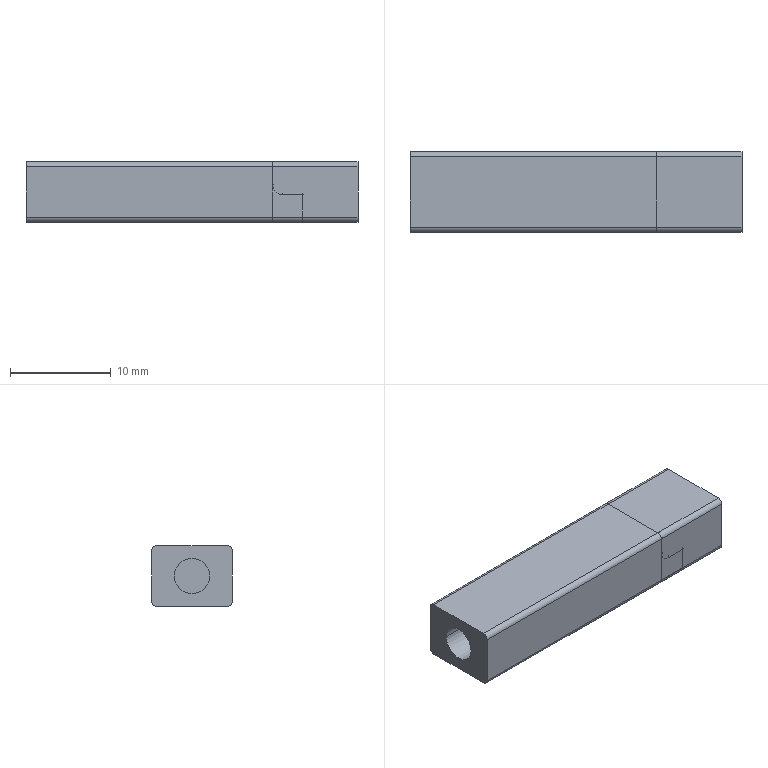NC program | NX | posted with a generic post | part box 33 x 8 x 6 mm
Lines 1 to 1894 of 11867, first 1555 of 1876 lines:
N10 G17 G21 G94 G90
(CAVITY_MILL_COPY , TOOL : D4)
N12 T04 M6
N14 G54
N16 G17 G0 G90 X2.078 Y5.8 B0. C0. S9500 M3
N18 G43 Z30. H4
N20 Z-0.445
N22 G94 G1 X0.866 Y3.7 F1000.
N24 G2 X0. Y3.2 R1.
N26 G1 X-3.5 F2000.
N28 G3 X-4.2 Y2.5 R0.7
N30 G1 Y-2.5
N32 G3 X-3.5 Y-3.2 R0.7
N34 G1 X-3.093
N36 G3 X-0.373 Y-4.42 R3.658
N38 X0.205 Y-5. R3.158
N40 G1 X1.429
N42 G2 X-0.087 Y-3.847 R2.598
N44 X2.14 Y1.058 R-3.098
N46 X5.731 Y-2. R3.098
N48 G1 Y-2.5
N50 G2 X3.996 Y-4.95 R2.598
N52 G3 X6. Y-2.5 R2.5
N54 G1 Y-0.569
N56 G3 X4.2 Y1.305 R3.658
N58 G1 Y2.5
N60 G3 X3.5 Y3.2 R0.7
N62 G1 X0.
N64 G2 X-0.866 Y3.7 R1.
N66 G1 X-2.078 Y5.8
N68 G0 X2.078 Z-0.891
N70 G1 X0.866 Y3.7 F1000.
N72 G2 X0. Y3.2 R1.
N74 G1 X-3.5 F2000.
N76 G3 X-4.2 Y2.5 R0.7
N78 G1 Y-2.5
N80 G3 X-3.5 Y-3.2 R0.7
N82 G1 X-3.096
N84 G3 X-0.374 Y-4.423 R3.66
N86 X0.201 Y-5. R3.16
N88 G1 X1.42
N90 G2 X-0.088 Y-3.85 R2.6
N92 X0.99 Y2.025 R-3.1
N94 X2.141 Y1.061 R3.1
N96 X5.734 Y-2. R3.1
N98 G1 Y-2.5
N100 G2 X4.014 Y-4.947 R2.6
N102 G3 X6. Y-2.5 R2.5
N104 G1 Y-0.563
N106 G3 X4.2 Y1.308 R3.66
N108 G1 Y2.5
N110 G3 X3.5 Y3.2 R0.7
N112 G1 X0.
N114 G2 X-0.866 Y3.7 R1.
N116 G1 X-2.078 Y5.8
N118 G0 X2.078 Z-1.336
N120 G1 X0.866 Y3.7 F1000.
N122 G2 X0. Y3.2 R1.
N124 G1 X-3.5 F2000.
N126 G3 X-4.2 Y2.5 R0.7
N128 G1 Y-2.5
N130 G3 X-3.5 Y-3.2 R0.7
N132 G1 X-3.096
N134 G3 X-0.374 Y-4.423 R3.66
N136 X0.201 Y-5. R3.16
N138 G1 X1.42
N140 G2 X-0.088 Y-3.85 R2.6
N142 X0.99 Y2.025 R-3.1
N144 X2.141 Y1.061 R3.1
N146 X5.734 Y-2. R3.1
N148 G1 Y-2.5
N150 G2 X4.014 Y-4.947 R2.6
N152 G3 X6. Y-2.5 R2.5
N154 G1 Y-0.563
N156 G3 X4.2 Y1.308 R3.66
N158 G1 Y2.5
N160 G3 X3.5 Y3.2 R0.7
N162 G1 X0.
N164 G2 X-0.866 Y3.7 R1.
N166 G1 X-2.078 Y5.8
N168 G0 X2.078 Z-1.782
N170 G1 X0.866 Y3.7 F1000.
N172 G2 X0. Y3.2 R1.
N174 G1 X-3.5 F2000.
N176 G3 X-4.2 Y2.5 R0.7
N178 G1 Y-2.5
N180 G3 X-3.5 Y-3.2 R0.7
N182 G1 X-3.096
N184 G3 X-0.374 Y-4.423 R3.66
N186 X0.201 Y-5. R3.16
N188 G1 X1.42
N190 G2 X-0.088 Y-3.85 R2.6
N192 X0.99 Y2.025 R-3.1
N194 X2.141 Y1.061 R3.1
N196 X5.734 Y-2. R3.1
N198 G1 Y-2.5
N200 G2 X4.014 Y-4.947 R2.6
N202 G3 X6. Y-2.5 R2.5
N204 G1 Y-0.563
N206 G3 X4.2 Y1.308 R3.66
N208 G1 Y2.5
N210 G3 X3.5 Y3.2 R0.7
N212 G1 X0.
N214 G2 X-0.866 Y3.7 R1.
N216 G1 X-2.078 Y5.8
N218 G0 X2.078 Z-2.227
N220 G1 X0.866 Y3.7 F1000.
N222 G2 X0. Y3.2 R1.
N224 G1 X-3.5 F2000.
N226 G3 X-4.2 Y2.5 R0.7
N228 G1 Y-2.5
N230 G3 X-3.5 Y-3.2 R0.7
N232 G1 X-3.096
N234 G3 X-0.374 Y-4.423 R3.66
N236 X0.201 Y-5. R3.16
N238 G1 X1.42
N240 G2 X-0.088 Y-3.85 R2.6
N242 X1.457 Y1.745 R-3.1
N244 X2.141 Y1.061 R3.1
N246 X5.734 Y-2. R3.1
N248 G1 Y-2.5
N250 G2 X4.014 Y-4.947 R2.6
N252 G3 X6. Y-2.5 R2.5
N254 G1 Y-0.563
N256 G3 X4.2 Y1.308 R3.66
N258 G1 Y2.5
N260 G3 X3.5 Y3.2 R0.7
N262 G1 X0.
N264 G2 X-0.866 Y3.7 R1.
N266 G1 X-2.078 Y5.8
N268 G0 X2.078 Z-2.673
N270 G1 X0.866 Y3.7 F1000.
N272 G2 X0. Y3.2 R1.
N274 G1 X-3.5 F2000.
N276 G3 X-4.2 Y2.5 R0.7
N278 G1 Y-2.5
N280 G3 X-3.5 Y-3.2 R0.7
N282 G1 X-3.096
N284 G3 X-0.374 Y-4.423 R3.66
N286 X0.201 Y-5. R3.16
N288 G1 X1.42
N290 G2 X-0.088 Y-3.85 R2.6
N292 X0.99 Y2.025 R-3.1
N294 X2.141 Y1.061 R3.1
N296 X5.734 Y-2. R3.1
N298 G1 Y-2.5
N300 G2 X4.014 Y-4.947 R2.6
N302 G3 X6. Y-2.5 R2.5
N304 G1 Y-0.563
N306 G3 X4.2 Y1.308 R3.66
N308 G1 Y2.5
N310 G3 X3.5 Y3.2 R0.7
N312 G1 X0.
N314 G2 X-0.866 Y3.7 R1.
N316 G1 X-2.078 Y5.8
N318 G0 X2.078 Z-3.118
N320 G1 X0.866 Y3.7 F1000.
N322 G2 X0. Y3.2 R1.
N324 G1 X-3.5 F2000.
N326 G3 X-4.2 Y2.5 R0.7
N328 G1 Y-2.5
N330 G3 X-3.5 Y-3.2 R0.7
N332 G1 X-3.096
N334 G3 X-0.374 Y-4.423 R3.66
N336 X0.201 Y-5. R3.16
N338 G1 X1.42
N340 G2 X-0.088 Y-3.85 R2.6
N342 X0.99 Y2.025 R-3.1
N344 X2.141 Y1.061 R3.1
N346 X5.734 Y-2. R3.1
N348 G1 Y-2.5
N350 G2 X4.014 Y-4.947 R2.6
N352 G3 X6. Y-2.5 R2.5
N354 G1 Y-0.563
N356 G3 X4.2 Y1.308 R3.66
N358 G1 Y2.5
N360 G3 X3.5 Y3.2 R0.7
N362 G1 X0.
N364 G2 X-0.866 Y3.7 R1.
N366 G1 X-2.078 Y5.8
N368 G0 X2.078 Z-3.564
N370 G1 X0.866 Y3.7 F1000.
N372 G2 X0. Y3.2 R1.
N374 G1 X-3.5 F2000.
N376 G3 X-4.2 Y2.5 R0.7
N378 G1 Y-2.5
N380 G3 X-3.5 Y-3.2 R0.7
N382 G1 X-3.096
N384 G3 X-0.374 Y-4.423 R3.66
N386 X0.201 Y-5. R3.16
N388 G1 X1.42
N390 G2 X-0.088 Y-3.85 R2.6
N392 X0.99 Y2.025 R-3.1
N394 X2.141 Y1.061 R3.1
N396 X5.734 Y-2. R3.1
N398 G1 Y-2.5
N400 G2 X4.014 Y-4.947 R2.6
N402 G3 X6. Y-2.5 R2.5
N404 G1 Y-0.563
N406 G3 X4.2 Y1.308 R3.66
N408 G1 Y2.5
N410 G3 X3.5 Y3.2 R0.7
N412 G1 X0.
N414 G2 X-0.866 Y3.7 R1.
N416 G1 X-2.078 Y5.8
N418 G0 X2.078 Z-4.009
N420 G1 X0.866 Y3.7 F1000.
N422 G2 X0. Y3.2 R1.
N424 G1 X-3.5 F2000.
N426 G3 X-4.2 Y2.5 R0.7
N428 G1 Y-2.5
N430 G3 X-3.5 Y-3.2 R0.7
N432 G1 X-3.096
N434 G3 X-0.374 Y-4.423 R3.66
N436 X0.201 Y-5. R3.16
N438 G1 X1.42
N440 G2 X-0.088 Y-3.85 R2.6
N442 X0.99 Y2.025 R-3.1
N444 X2.142 Y1.061 R3.1
N446 X5.734 Y-2. R3.1
N448 G1 Y-2.5
N450 G2 X4.014 Y-4.947 R2.6
N452 G3 X6. Y-2.5 R2.5
N454 G1 Y-0.563
N456 G3 X4.2 Y1.308 R3.66
N458 G1 Y2.5
N460 G3 X3.5 Y3.2 R0.7
N462 G1 X0.
N464 G2 X-0.866 Y3.7 R1.
N466 G1 X-2.078 Y5.8
N468 G0 X2.078 Z-4.455
N470 G1 X0.866 Y3.7 F1000.
N472 G2 X0. Y3.2 R1.
N474 G1 X-3.5 F2000.
N476 G3 X-4.2 Y2.5 R0.7
N478 G1 Y-2.5
N480 G3 X-3.5 Y-3.2 R0.7
N482 G1 X-3.096
N484 G3 X-0.374 Y-4.423 R3.66
N486 X0.201 Y-5. R3.16
N488 G1 X1.42
N490 G2 X-0.088 Y-3.85 R2.6
N492 X0.99 Y2.025 R-3.1
N494 X2.142 Y1.061 R3.1
N496 X5.734 Y-2. R3.1
N498 G1 Y-2.5
N500 G2 X4.014 Y-4.947 R2.6
N502 G3 X6. Y-2.5 R2.5
N504 G1 Y-0.563
N506 G3 X4.2 Y1.308 R3.66
N508 G1 Y2.5
N510 G3 X3.5 Y3.2 R0.7
N512 G1 X0.
N514 G2 X-0.866 Y3.7 R1.
N516 G1 X-2.078 Y5.8
N518 G0 X2.078 Z-4.9
N520 G1 X0.866 Y3.7 F1000.
N522 G2 X0. Y3.2 R1.
N524 G1 X-3.5 F2000.
N526 G3 X-4.2 Y2.5 R0.7
N528 G1 Y0.316
N530 G3 X-4.2 Y-1.842 R3.983
N532 G1 Y-2.5
N534 G3 X-3.516 Y-3.2 R0.7
N536 X-0.27 Y-4.744 R3.983
N538 X0.044 Y-5. R3.518
N540 G1 X1.318
N542 G2 X-0.054 Y-4.171 R2.958
N544 X-3.537 Y0.526 R3.423
N546 X-1.61 Y2.188 R3.108
N548 G1 X-0.872 Y2.334
N550 X-0.826 Y2.353
N552 X-0.812 Y2.305
N554 G2 X0.106 Y2.301 R3.1
N556 G1 X0.141 Y2.329
N558 G2 X2.214 Y1.397 R3.365
N560 X4.793 Y0.656 R3.423
N562 X5.964 Y-2. R3.378
N564 G1 Y-2.5
N566 G2 X5.151 Y-4.328 R2.464
N568 X4.409 Y-4.829 R2.844
N570 G3 X6. Y-2.5 R2.5
N572 G1 Y0.063
N574 G3 X5.147 Y1.09 R3.938
N576 X4.2 Y1.662 R3.983
N578 G1 Y2.5
N580 G3 X3.5 Y3.2 R0.7
N582 G1 X0.
N584 G2 X-0.866 Y3.7 R1.
N586 G1 X-2.078 Y5.8
N588 G0 X2.078 Z-5.329
N590 G1 X0.866 Y3.7 F1000.
N592 G2 X0. Y3.2 R1.
N594 G1 X-3.5 F2000.
N596 G3 X-4.128 Y2.809 R0.7
N598 X-6. Y1.629 R3.135
N600 G1 Y0.354
N602 G2 X-3.5 Y2.312 R2.575
N604 G1 X-1.858
N606 X-1.169 Y2.337
N608 X0.432
N610 X0.516 Y2.335
N612 X0.99 Y2.294
N614 X1.052 Y2.312
N616 X3.5
N618 G2 X6. Y0.354 R2.575
N620 G1 Y1.629
N622 G3 X4.128 Y2.809 R3.135
N624 X3.5 Y3.2 R0.7
N626 G1 X0.
N628 G2 X-0.866 Y3.7 R1.
N630 G1 X-2.078 Y5.8
N632 G0 X2.078 Z-5.757
N634 G1 X0.866 Y3.7 F1000.
N636 G2 X0. Y3.2 R1.
N638 G1 X-3.5 F2000.
N640 G3 X-4.113 Y2.837 R0.7
N642 X-6. Y1.67 R3.16
N644 G1 Y0.452
N646 G2 X-3.5 Y2.337 R2.6
N648 G1 X3.5
N650 G2 X6. Y0.452 R2.6
N652 G1 Y1.67
N654 G3 X4.113 Y2.837 R3.16
N656 X3.5 Y3.2 R0.7
N658 G1 X0.
N660 G2 X-0.866 Y3.7 R1.
N662 G1 X-2.078 Y5.8
N664 G0 X2.078 Z-6.186
N666 G1 X0.866 Y3.7 F1000.
N668 G2 X0. Y3.2 R1.
N670 G1 X-3.5 F2000.
N672 G3 X-4.113 Y2.837 R0.7
N674 X-6. Y1.67 R3.16
N676 G1 Y0.452
N678 G2 X-3.5 Y2.337 R2.6
N680 G1 X3.5
N682 G2 X6. Y0.452 R2.6
N684 G1 Y1.67
N686 G3 X4.113 Y2.837 R3.16
N688 X3.5 Y3.2 R0.7
N690 G1 X0.
N692 G2 X-0.866 Y3.7 R1.
N694 G1 X-2.078 Y5.8
N696 G0 X2.078 Z-6.614
N698 G1 X0.866 Y3.7 F1000.
N700 G2 X0. Y3.2 R1.
N702 G1 X-3.5 F2000.
N704 G3 X-4.113 Y2.837 R0.7
N706 X-6. Y1.67 R3.16
N708 G1 Y0.452
N710 G2 X-3.5 Y2.337 R2.6
N712 G1 X3.5
N714 G2 X6. Y0.452 R2.6
N716 G1 Y1.67
N718 G3 X4.113 Y2.837 R3.16
N720 X3.5 Y3.2 R0.7
N722 G1 X0.
N724 G2 X-0.866 Y3.7 R1.
N726 G1 X-2.078 Y5.8
N728 G0 X2.078 Z-7.043
N730 G1 X0.866 Y3.7 F1000.
N732 G2 X0. Y3.2 R1.
N734 G1 X-3.5 F2000.
N736 G3 X-4.113 Y2.837 R0.7
N738 X-6. Y1.67 R3.16
N740 G1 Y0.452
N742 G2 X-3.5 Y2.337 R2.6
N744 G1 X3.5
N746 G2 X6. Y0.452 R2.6
N748 G1 Y1.67
N750 G3 X4.113 Y2.837 R3.16
N752 X3.5 Y3.2 R0.7
N754 G1 X0.
N756 G2 X-0.866 Y3.7 R1.
N758 G1 X-2.078 Y5.8
N760 G0 X2.078 Z-7.471
N762 G1 X0.866 Y3.7 F1000.
N764 G2 X0. Y3.2 R1.
N766 G1 X-3.5 F2000.
N768 G3 X-4.113 Y2.837 R0.7
N770 X-6. Y1.67 R3.16
N772 G1 Y0.452
N774 G2 X-3.5 Y2.337 R2.6
N776 G1 X3.5
N778 G2 X6. Y0.452 R2.6
N780 G1 Y1.67
N782 G3 X4.113 Y2.837 R3.16
N784 X3.5 Y3.2 R0.7
N786 G1 X0.
N788 G2 X-0.866 Y3.7 R1.
N790 G1 X-2.078 Y5.8
N792 G0 X2.056 Z-7.9
N794 G1 X0.856 Y3.72 F1000.
N796 G2 X-0.01 Y3.22 R1.
N798 G1 X-3.545 Y3.219 F2000.
N800 G3 X-6. Y1.846 R3.375
N802 G1 Y0.563
N804 G2 X-3.5 Y2.66 R2.815
N806 G1 X3.5
N808 G2 X5.602 Y1.409 R2.579
N810 X6. Y0.601 R2.569
N812 G1 Y1.827
N814 G3 X3.5 Y3.22 R3.139
N816 G1 X-0.01
N818 G2 X-0.876 Y3.72 R1.
N820 G1 X-2.077 Y5.8
N822 G0 Z30.
(ZLEVEL_PROFILE_COPY_COPY_COPY , TOOL : D4)
N824 X-6.742 Y-3.115
N826 Z-6.
N828 G1 Z-7.5 F1000.
N830 X-6.198 Y-2.802
N832 G3 X-5.998 Y-2.455 R0.4
N834 G1 Y-0.834 F1200.
N836 X-6. Y-0.556
N838 Y-0.263
N840 G2 X-3.5 Y2.237 R2.5
N842 G1 X3.5
N844 G2 X6. Y-0.263 R2.5
N846 G1 Y-0.556
N848 X5.999 Y-0.834
N850 Y-2.455
N852 G3 X6.2 Y-2.802 R0.4
N854 G1 X6.742 Y-3.115
N856 Z-6.
N858 G0 Z30.
(FLOOR_WALL_1 , TOOL : D4)
N860 X-6.903 Y5.03
N862 Z-6.5
N864 G1 Z-8. F1000.
N866 X-5.846 Y3.199
N868 G3 X-5.5 Y2.999 R0.4
N870 G1 X5.5
N872 G3 X5.846 Y3.199 R0.4
N874 G1 X6.903 Y5.03
N876 Z-6.5
N878 G0 Z30.
N880 M5
(CAVITY_MILL_COPY_COPY , TOOL : D2)
N882 T12 M6
N884 G54
N886 G17 G0 G90 X0.856 Y1.186 B0. C0. S9500 M3
N888 G43 Z30. H12
N890 Z-0.2
N892 G94 G3 X1.087 Y0.461 R1. F1000.
N894 G2 X1.511 Y-0.467 R1.9
N896 X2.466 Y-0.107 R1.9
N898 G3 X3.141 Y0.243 R1.
N900 G0 X0.897 Y1.266 Z-0.4
N902 G3 X1.138 Y0.54 R1.
N904 G2 X1.573 Y-0.316 R1.99
N906 X2.485 Y-0.016 R1.99
N908 G3 X3.169 Y0.329 R1.
N910 G0 X0.902 Y1.275 Z-0.6
N912 G3 X1.144 Y0.549 R1.
N914 G2 X1.58 Y-0.3 R2.
N916 X2.488 Y-0.005 R2.
N918 G3 X3.172 Y0.339 R1.
N920 G0 X0.902 Y1.275 Z-0.8
N922 G3 X1.144 Y0.549 R1.
N924 G2 X1.58 Y-0.3 R2.
N926 X2.488 Y-0.005 R2.
N928 G3 X3.172 Y0.339 R1.
N930 G0 X0.902 Y1.275 Z-1.
N932 G3 X1.144 Y0.549 R1.
N934 G2 X1.58 Y-0.3 R2.
N936 X2.488 Y-0.005 R2.
N938 G3 X3.172 Y0.339 R1.
N940 G0 X0.902 Y1.275 Z-1.2
N942 G3 X1.144 Y0.549 R1.
N944 G2 X1.58 Y-0.3 R2.
N946 X2.488 Y-0.005 R2.
N948 G3 X3.172 Y0.339 R1.
N950 G0 X0.902 Y1.275 Z-1.4
N952 G3 X1.144 Y0.549 R1.
N954 G2 X1.58 Y-0.3 R2.
N956 X2.488 Y-0.005 R2.
N958 G3 X3.172 Y0.339 R1.
N960 G0 X0.902 Y1.275 Z-1.6
N962 G3 X1.144 Y0.549 R1.
N964 G2 X1.58 Y-0.3 R2.
N966 X2.488 Y-0.005 R2.
N968 G3 X3.172 Y0.339 R1.
N970 G0 X0.902 Y1.275 Z-1.8
N972 G3 X1.144 Y0.549 R1.
N974 G2 X1.58 Y-0.3 R2.
N976 X2.488 Y-0.005 R2.
N978 G3 X3.172 Y0.339 R1.
N980 G0 X0.902 Y1.275 Z-2.
N982 G3 X1.144 Y0.549 R1.
N984 G2 X1.58 Y-0.3 R2.
N986 X2.488 Y-0.005 R2.
N988 G3 X3.172 Y0.339 R1.
N990 G0 X0.902 Y1.275 Z-2.2
N992 G3 X1.144 Y0.549 R1.
N994 G2 X1.58 Y-0.3 R2.
N996 X2.488 Y-0.005 R2.
N998 G3 X3.172 Y0.339 R1.
N1000 G0 X0.902 Y1.275 Z-2.4
N1002 G3 X1.144 Y0.549 R1.
N1004 G2 X1.58 Y-0.3 R2.
N1006 X2.488 Y-0.005 R2.
N1008 G3 X3.172 Y0.339 R1.
N1010 G0 X0.902 Y1.275 Z-2.6
N1012 G3 X1.144 Y0.549 R1.
N1014 G2 X1.58 Y-0.3 R2.
N1016 X2.488 Y-0.005 R2.
N1018 G3 X3.172 Y0.339 R1.
N1020 G0 X0.902 Y1.275 Z-2.8
N1022 G3 X1.144 Y0.549 R1.
N1024 G2 X1.58 Y-0.3 R2.
N1026 X2.488 Y-0.005 R2.
N1028 G3 X3.172 Y0.339 R1.
N1030 G0 X0.902 Y1.275 Z-3.
N1032 G3 X1.144 Y0.549 R1.
N1034 G2 X1.58 Y-0.3 R2.
N1036 X2.488 Y-0.005 R2.
N1038 G3 X3.172 Y0.339 R1.
N1040 G0 X0.902 Y1.275 Z-3.2
N1042 G3 X1.144 Y0.549 R1.
N1044 G2 X1.58 Y-0.3 R2.
N1046 X2.488 Y-0.005 R2.
N1048 G3 X3.172 Y0.339 R1.
N1050 G0 X0.902 Y1.275 Z-3.4
N1052 G3 X1.144 Y0.549 R1.
N1054 G2 X1.58 Y-0.3 R2.
N1056 X2.488 Y-0.005 R2.
N1058 G3 X3.172 Y0.339 R1.
N1060 G0 X0.902 Y1.275 Z-3.6
N1062 G3 X1.144 Y0.549 R1.
N1064 G2 X1.58 Y-0.3 R2.
N1066 X2.488 Y-0.005 R2.
N1068 G3 X3.172 Y0.339 R1.
N1070 G0 X0.902 Y1.275 Z-3.8
N1072 G3 X1.144 Y0.549 R1.
N1074 G2 X1.58 Y-0.3 R2.
N1076 X2.488 Y-0.005 R2.
N1078 G3 X3.172 Y0.339 R1.
N1080 G0 X0.902 Y1.275 Z-4.
N1082 G3 X1.144 Y0.549 R1.
N1084 G2 X1.58 Y-0.3 R2.
N1086 X2.488 Y-0.005 R2.
N1088 G3 X3.172 Y0.339 R1.
N1090 G0 X0.902 Y1.275 Z-4.2
N1092 G3 X1.144 Y0.549 R1.
N1094 G2 X1.58 Y-0.3 R2.
N1096 X2.488 Y-0.005 R2.
N1098 G3 X3.172 Y0.339 R1.
N1100 G0 X0.902 Y1.275 Z-4.4
N1102 G3 X1.144 Y0.549 R1.
N1104 G2 X1.58 Y-0.3 R2.
N1106 X2.488 Y-0.005 R2.
N1108 G3 X3.172 Y0.339 R1.
N1110 G0 X0.906 Y1.284 Z-4.6
N1112 G3 X1.15 Y0.558 R1.
N1114 G2 X1.586 Y-0.284 R2.01
N1116 X2.49 Y0.005 R2.01
N1118 G3 X3.175 Y0.349 R1.
N1120 G0 X0.947 Y1.358 Z-4.8
N1122 G3 X1.2 Y0.637 R1.
N1124 G2 X1.642 Y-0.149 R2.1
N1126 X2.51 Y0.096 R2.1
N1128 G3 X3.203 Y0.434 R1.
N1130 G0 X0.899 Y1.476 Z-5.
N1132 G3 X1.292 Y0.81 R1.
N1134 G2 X1.803 Y0.266 R2.15
N1136 X2.521 Y0.411 R2.414
N1138 G3 X3.226 Y0.751 R1.
N1140 G0 Z30.
N1142 X1.235 Y-4.059
N1144 Z-0.2
N1146 G3 X1.028 Y-3.359 R1.
N1148 G2 X0.734 Y-2.5 R1.4
N1150 G1 Y-2.312
N1152 G2 X-0.329 Y-2.662 R1.9
N1154 G3 X-1.027 Y-2.966 R1.
N1156 G0 X1.183 Y-4.133 Z-0.4
N1158 G3 X0.969 Y-3.428 R1.
N1160 G2 X0.644 Y-2.477 R1.49
N1162 X-0.355 Y-2.752 R1.99
N1164 G3 X-1.061 Y-3.049 R1.
N1166 G0 X1.177 Y-4.142 Z-0.6
N1168 G3 X0.962 Y-3.436 R1.
N1170 G2 X0.634 Y-2.495 R1.5
N1172 X-0.359 Y-2.763 R2.
N1174 G3 X-1.065 Y-3.059 R1.
N1176 G0 X1.177 Y-4.142 Z-0.8
N1178 G3 X0.962 Y-3.436 R1.
N1180 G2 X0.634 Y-2.495 R1.5
N1182 X-0.359 Y-2.763 R2.
N1184 G3 X-1.065 Y-3.059 R1.
N1186 G0 X1.177 Y-4.142 Z-1.
N1188 G3 X0.962 Y-3.436 R1.
N1190 G2 X0.634 Y-2.495 R1.5
N1192 X-0.359 Y-2.763 R2.
N1194 G3 X-1.065 Y-3.059 R1.
N1196 G0 X1.177 Y-4.142 Z-1.2
N1198 G3 X0.962 Y-3.436 R1.
N1200 G2 X0.634 Y-2.495 R1.5
N1202 X-0.359 Y-2.763 R2.
N1204 G3 X-1.065 Y-3.059 R1.
N1206 G0 X1.177 Y-4.142 Z-1.4
N1208 G3 X0.962 Y-3.436 R1.
N1210 G2 X0.634 Y-2.495 R1.5
N1212 X-0.359 Y-2.763 R2.
N1214 G3 X-1.065 Y-3.059 R1.
N1216 G0 X1.177 Y-4.142 Z-1.6
N1218 G3 X0.962 Y-3.436 R1.
N1220 G2 X0.634 Y-2.495 R1.5
N1222 X-0.359 Y-2.763 R2.
N1224 G3 X-1.065 Y-3.059 R1.
N1226 G0 X1.177 Y-4.142 Z-1.8
N1228 G3 X0.962 Y-3.436 R1.
N1230 G2 X0.634 Y-2.495 R1.5
N1232 X-0.359 Y-2.763 R2.
N1234 G3 X-1.065 Y-3.059 R1.
N1236 G0 X1.177 Y-4.142 Z-2.
N1238 G3 X0.962 Y-3.436 R1.
N1240 G2 X0.634 Y-2.495 R1.5
N1242 X-0.359 Y-2.763 R2.
N1244 G3 X-1.065 Y-3.059 R1.
N1246 G0 X1.177 Y-4.142 Z-2.2
N1248 G3 X0.962 Y-3.436 R1.
N1250 G2 X0.634 Y-2.495 R1.5
N1252 X-0.359 Y-2.763 R2.
N1254 G3 X-1.065 Y-3.059 R1.
N1256 G0 X1.177 Y-4.142 Z-2.4
N1258 G3 X0.962 Y-3.436 R1.
N1260 G2 X0.634 Y-2.495 R1.5
N1262 X-0.359 Y-2.763 R2.
N1264 G3 X-1.065 Y-3.059 R1.
N1266 G0 X1.177 Y-4.142 Z-2.6
N1268 G3 X0.962 Y-3.436 R1.
N1270 G2 X0.634 Y-2.495 R1.5
N1272 X-0.359 Y-2.763 R2.
N1274 G3 X-1.065 Y-3.059 R1.
N1276 G0 X1.177 Y-4.142 Z-2.8
N1278 G3 X0.962 Y-3.436 R1.
N1280 G2 X0.634 Y-2.495 R1.5
N1282 X-0.359 Y-2.763 R2.
N1284 G3 X-1.065 Y-3.059 R1.
N1286 G0 X1.177 Y-4.142 Z-3.
N1288 G3 X0.962 Y-3.436 R1.
N1290 G2 X0.634 Y-2.495 R1.5
N1292 X-0.359 Y-2.763 R2.
N1294 G3 X-1.065 Y-3.059 R1.
N1296 G0 X1.177 Y-4.142 Z-3.2
N1298 G3 X0.962 Y-3.436 R1.
N1300 G2 X0.634 Y-2.495 R1.5
N1302 X-0.359 Y-2.763 R2.
N1304 G3 X-1.065 Y-3.059 R1.
N1306 G0 X1.177 Y-4.142 Z-3.4
N1308 G3 X0.962 Y-3.436 R1.
N1310 G2 X0.634 Y-2.495 R1.5
N1312 X-0.359 Y-2.763 R2.
N1314 G3 X-1.065 Y-3.059 R1.
N1316 G0 X1.177 Y-4.142 Z-3.6
N1318 G3 X0.962 Y-3.436 R1.
N1320 G2 X0.634 Y-2.495 R1.5
N1322 X-0.359 Y-2.763 R2.
N1324 G3 X-1.065 Y-3.059 R1.
N1326 G0 X1.177 Y-4.142 Z-3.8
N1328 G3 X0.962 Y-3.436 R1.
N1330 G2 X0.634 Y-2.495 R1.5
N1332 X-0.359 Y-2.763 R2.
N1334 G3 X-1.065 Y-3.059 R1.
N1336 G0 X1.177 Y-4.142 Z-4.
N1338 G3 X0.962 Y-3.436 R1.
N1340 G2 X0.634 Y-2.495 R1.5
N1342 X-0.359 Y-2.763 R2.
N1344 G3 X-1.065 Y-3.059 R1.
N1346 G0 X1.177 Y-4.142 Z-4.2
N1348 G3 X0.962 Y-3.436 R1.
N1350 G2 X0.634 Y-2.495 R1.5
N1352 X-0.359 Y-2.763 R2.
N1354 G3 X-1.065 Y-3.059 R1.
N1356 G0 X1.177 Y-4.142 Z-4.4
N1358 G3 X0.962 Y-3.436 R1.
N1360 G2 X0.634 Y-2.495 R1.5
N1362 X-0.359 Y-2.763 R2.
N1364 G3 X-1.065 Y-3.059 R1.
N1366 G0 X1.175 Y-4.14 Z-4.6
N1368 G3 X0.949 Y-3.432 R1.
N1370 G2 X0.62 Y-2.514 R1.436
N1372 X-0.361 Y-2.773 R2.01
N1374 G3 X-1.068 Y-3.068 R1.
N1376 G0 X1.172 Y-4.183 Z-4.8
N1378 G3 X0.917 Y-3.49 R1.
N1380 G2 X0.543 Y-2.656 R1.501
N1382 X-0.375 Y-2.863 R2.1
N1384 G3 X-1.087 Y-3.156 R1.
N1386 G0 X1.198 Y-4.238 Z-5.
N1388 G3 X0.822 Y-3.568 R1.
N1390 G2 X0.363 Y-3.064 R2.058
N1392 X-0.32 Y-3.176 R2.414
N1394 G3 X-1.035 Y-3.496 R1.
N1396 G0 Z30.
(ZLEVEL_PROFILE_COPY_1_COPY_COPY , TOOL : D2)
N1398 X-5.4 Y-1.169
N1400 Z-6.05
N1402 G1 Z-7.55
N1404 X-5.101 Y-0.997
N1406 G3 X-5. Y-0.825 R0.2
N1408 G1 X-4.998 Y-0.245 F1500.
N1410 G2 X-3.5 Y1.24 R1.496
N1412 G1 X3.5
N1414 G2 X3.937 Y1.171 R1.147
N1416 X4.999 Y-0.245 R1.487
N1418 G1 X5. Y-0.825
N1420 Z-7.599
N1422 X4.999 Y-0.245
N1424 G3 X3.937 Y1.184 R1.5
N1426 X3.544 Y1.254 R1.296
N1428 G1 X3.5 Y1.247
N1430 X-3.5
N1432 G3 X-3.741 Y1.235 R2.815
N1434 G1 X-3.937 Y1.184
N1436 G3 X-4.998 Y-0.245 R1.496
N1438 G1 X-5. Y-0.825
N1440 Z-7.648
N1442 X-4.998 Y-0.245
N1444 G2 X-3.5 Y1.26 R1.49
N1446 G1 X3.5
N1448 G2 X4.986 Y-0.052 R1.489
N1450 X5. Y-0.825 R9.913
N1452 G1 Z-7.694
N1454 X4.999 Y-0.245
N1456 G3 X3.5 Y1.277 R1.505
N1458 G1 X-3.5
N1460 G3 X-4.998 Y-0.245 R1.502
N1462 G1 X-5. Y-0.825
N1464 Z-7.739
N1466 X-4.998 Y-0.245
N1468 G2 X-3.496 Y1.298 R1.513
N1470 G1 X3.496
N1472 G2 X4.999 Y-0.245 R1.516
N1474 G1 X5. Y-0.825
N1476 Z-7.781
N1478 G3 X4.992 Y-0.108 R12.542
N1480 X4.681 Y0.72 R1.413
N1482 X3.5 Y1.324 R1.458
N1484 G1 X-3.5
N1486 X-3.544 Y1.333
N1488 G3 X-4.998 Y-0.245 R1.546
N1490 G1 X-5. Y-0.825
N1492 Z-7.821
N1494 X-4.998 Y-0.186
N1496 G2 X-3.625 Y1.353 R1.555
N1498 G1 X-3.544 Y1.363
N1500 X-3.5 Y1.354
N1502 X3.501
N1504 G2 X4.163 Y1.188 R1.407
N1506 X4.999 Y-0.245 R1.581
N1508 G1 X5. Y-0.825
N1510 Z-7.857
N1512 X4.999 Y-0.245
N1514 G3 X4.274 Y1.154 R1.625
N1516 X3.501 Y1.387 R1.397
N1518 G1 X-3.549
N1520 G3 X-3.959 Y1.312 R1.157
N1522 X-4.998 Y-0.186 R1.608
N1524 G1 X-5. Y-0.825
N1526 Z-7.889
N1528 X-4.998 Y-0.245
N1530 X-4.995 Y-0.136
N1532 G2 X-4.134 Y1.271 R1.649
N1534 X-3.536 Y1.423 R1.252
N1536 G1 X3.501
N1538 G2 X4.308 Y1.162 R1.377
N1540 X4.999 Y-0.245 R1.673
N1542 G1 X5. Y-0.825
N1544 Z-7.917
N1546 X4.999 Y-0.171
N1548 G3 X4.221 Y1.251 R1.691
N1550 X3.501 Y1.462 R1.335
N1552 G1 X-3.5
N1554 G3 X-4.065 Y1.336 R1.192
N1556 X-4.998 Y-0.167 R1.688
N1558 G1 X-5. Y-0.825
N1560 Z-7.941
N1562 X-4.998 Y-0.166
N1564 G2 X-4.151 Y1.326 R1.75
N1566 X-3.5 Y1.502 R1.224
N1568 G1 X3.5
N1570 G2 X4.18 Y1.308 R1.287
N1572 X4.999 Y-0.164 R1.736
N1574 G1 X5. Y-0.825
N1576 Z-7.96
N1578 X4.999 Y-0.176
N1580 G3 X4.239 Y1.304 R1.824
N1582 X3.501 Y1.541 R1.265
N1584 G1 X-3.5
N1586 G3 X-4.183 Y1.342 R1.209
N1588 X-4.997 Y-0.149 R1.813
N1590 G1 X-4.998 Y-0.245
N1592 X-5. Y-0.825
N1594 Z-7.973
N1596 X-4.998 Y-0.162
N1598 G2 X-4.111 Y1.409 R1.845
N1600 X-3.5 Y1.574 R1.139
N1602 G1 X3.5
N1604 G2 X4.284 Y1.297 R1.287
N1606 X4.999 Y-0.178 R1.883
N1608 G1 X5. Y-0.825
N1610 Z-7.981
N1612 X4.999 Y-0.245
N1614 X4.996 Y-0.052
N1616 G3 X4.169 Y1.395 R1.906
N1618 X3.501 Y1.6 R1.186
N1620 G1 X-3.502
N1622 G3 X-4.152 Y1.405 R1.179
N1624 X-4.997 Y-0.156 R1.883
N1626 G1 X-5. Y-0.825
N1628 Z-7.987
N1630 X-4.997 Y-0.158
N1632 G2 X-4.311 Y1.299 R1.912
N1634 G1 X-4.23 Y1.367
N1636 G2 X-3.523 Y1.622 R1.108
N1638 G1 X3.561
N1640 G2 X4.201 Y1.391 R1.002
N1642 G1 X4.307 Y1.303
N1644 G2 X4.997 Y-0.158 R1.91
N1646 G1 X5. Y-0.825
N1648 Z-8.
N1650 X4.997 Y-0.15
N1652 G3 X4.46 Y1.177 R1.925
N1654 G1 X4.331 Y1.31
N1656 G3 X3.5 Y1.688 R1.158
N1658 G1 X-3.5
N1660 G3 X-4.341 Y1.299 R1.137
N1662 X-4.996 Y-0.052 R2.008
N1664 G1 X-5. Y-0.825
N1666 G2 X-5.101 Y-0.997 R0.2
N1668 G1 X-5.4 Y-1.168
N1670 Z-6.5
N1672 G0 Z30.
(ZLEVEL_PROFILE_COPY_1_COPY_COPY_COPY_1 , TOOL : D2)
N1674 Y-1.022
N1676 Z-6.51
N1678 G1 Z-8.01 F1000.
N1680 X-5.1 Y-0.852
N1682 G3 X-4.999 Y-0.68 R0.2
N1684 G1 X-4.995 Y-0.119 F1500.
N1686 G2 X-4.599 Y1.029 R1.907
N1688 G1 Y2.5
N1690 G2 X-3.5 Y3.599 R1.099
N1692 G1 X3.5
N1694 G2 X4.599 Y2.5 R1.099
N1696 G1 Y1.028
N1698 G2 X5. Y-0.192 R1.945
N1700 G1 Y-0.681
N1702 Y-0.669 Z-8.025
N1704 Y-0.192
N1706 G3 X4.655 Y0.969 R1.974
N1708 G1 Y2.5
N1710 G3 X3.5 Y3.655 R1.155
N1712 G1 X-3.5
N1714 G3 X-4.655 Y2.5 R1.155
N1716 G1 Y0.969
N1718 G3 X-4.995 Y-0.107 R1.914
N1720 G1 X-4.999 Y-0.668
N1722 Z-8.044
N1724 X-4.996 Y-0.134
N1726 G2 X-4.705 Y0.932 R2.143
N1728 G1 Y2.5
N1730 G2 X-3.5 Y3.705 R1.205
N1732 G1 X3.5
N1734 G2 X4.705 Y2.5 R1.205
N1736 G1 Y0.932
N1738 G2 X4.996 Y-0.126 R2.123
N1740 G1 X5. Y-0.669
N1742 Y-0.657 Z-8.067
N1744 Y-0.591
N1746 X4.997 Y-0.107
N1748 G3 X4.751 Y0.879 R2.154
N1750 G1 Y2.5
N1752 G3 X3.5 Y3.751 R1.251
N1754 G1 X-3.5
N1756 G3 X-4.751 Y2.5 R1.251
N1758 G1 Y0.879
N1760 G3 X-4.997 Y-0.11 R2.152
N1762 G1 X-4.999 Y-0.656
N1764 Y-0.644 Z-8.095
N1766 X-4.998 Y-0.116
N1768 G2 X-4.794 Y0.835 R2.352
N1770 G1 Y2.5
N1772 G2 X-3.5 Y3.794 R1.294
N1774 G1 X3.5
N1776 G2 X4.794 Y2.5 R1.294
N1778 G1 Y0.835
N1780 G2 X4.998 Y-0.105 R2.314
N1782 G1 X5. Y-0.645
N1784 Y-0.633 Z-8.127
N1786 Y-0.192
N1788 G3 X4.833 Y0.795 R2.633
N1790 G1 Y2.5
N1792 G3 X3.5 Y3.833 R1.333
N1794 G1 X-3.5
N1796 G3 X-4.833 Y2.5 R1.333
N1798 G1 Y0.79
N1800 G3 X-4.998 Y-0.09 R2.478
N1802 G1 X-4.999 Y-0.633
N1804 Y-0.609 Z-8.163
N1806 X-4.998 Y-0.102
N1808 G2 X-4.869 Y0.77 R3.083
N1810 G1 Y2.5
N1812 G2 X-3.5 Y3.869 R1.369
N1814 G1 X3.5
N1816 G2 X4.869 Y2.5 R1.369
N1818 G1 Y0.759
N1820 G2 X5. Y-0.192 R3.014
N1822 G1 Y-0.609
N1824 Y-0.597 Z-8.202
N1826 Y-0.192
N1828 G3 X4.902 Y0.737 R3.758
N1830 G1 Y2.5
N1832 G3 X3.5 Y3.902 R1.402
N1834 G1 X-3.5
N1836 G3 X-4.902 Y2.5 R1.402
N1838 G1 Y0.737
N1840 G3 X-4.998 Y-0.084 R3.637
N1842 G1 X-4.999 Y-0.597
N1844 Y-0.572 Z-8.244
N1846 X-4.992 Y0.208
N1848 X-4.93 Y0.737
N1850 Y2.5
N1852 G2 X-3.5 Y3.93 R1.43
N1854 G1 X3.5
N1856 G2 X4.93 Y2.5 R1.43
N1858 G1 Y0.737
N1860 G2 X5. Y-0.572 R7.106
N1862 G1 Y-0.547 Z-8.288
N1864 G3 X4.953 Y0.737 R10.411
N1866 G1 Y2.5
N1868 G3 X3.5 Y3.953 R1.453
N1870 G1 X-3.5
N1872 G3 X-4.953 Y2.5 R1.453
N1874 G1 Y0.737
N1876 G3 X-4.999 Y-0.547 R10.207
N1878 G1 Y-0.51 Z-8.335
N1880 G2 X-4.972 Y0.737 R18.981
N1882 G1 Y2.5
N1884 G2 X-3.5 Y3.972 R1.472
N1886 G1 X3.5
N1888 G2 X4.972 Y2.5 R1.472
N1890 G1 Y0.737
N1892 G2 X5. Y-0.51 R17.262
N1894 G1 Y-0.485 Z-8.376
N1896 G3 X4.984 Y0.737 R36.974
N1898 G1 Y2.5
N1900 G3 X3.5 Y3.984 R1.484
N1902 G1 X-3.5
N1904 G3 X-4.984 Y2.5 R1.484
N1906 G1 Y0.737
N1908 G3 X-4.999 Y-0.485 R48.45
N1910 G1 Y-0.46 Z-8.417
N1912 G3 X-4.993 Y0.737 R372.496
N1914 G1 Y2.5
N1916 G2 X-3.5 Y3.993 R1.493
N1918 G1 X3.5
N1920 G2 X4.993 Y2.5 R1.493
N1922 G1 Y0.737
N1924 X4.985 Y0.728
N1926 X4.99 Y0.607
N1928 X4.997 Y0.407
N1930 X5. Y-0.46
N1932 Y-0.423 Z-8.459
N1934 X4.998 Y0.737
N1936 Y2.5
N1938 G3 X3.5 Y3.998 R1.498
N1940 G1 X-3.5
N1942 G3 X-4.998 Y2.5 R1.498
N1944 G1 Y0.737
N1946 X-4.997 Y0.607
N1948 X-4.999 Y-0.423
N1950 Y-0.385 Z-8.5
N1952 X-4.997 Y0.607
N1954 X-4.998 Y0.737
N1956 X-4.999 Y2.51
N1958 X-4.994 Y2.668
N1960 G2 X-4.178 Y3.837 R1.516
N1962 X-3.504 Y3.998 R1.481
N1964 G1 X3.501 Y3.999
N1966 G2 X4.109 Y3.865 R1.446
N1968 X4.766 Y3.298 R1.426
N1970 X5. Y2.5 R1.469
N1972 G1 Y-0.192
N1974 Y-0.385
N1976 G3 X5.1 Y-0.558 R0.2
N1978 G1 X5.4 Y-0.731
N1980 Z-7.
N1982 G0 Z30.
(FLOOR_WALL_1_COPY , TOOL : D2)
N1984 X6.497 Y-2.129
N1986 Z-3.5
N1988 G1 Z-5. F1000.
N1990 X5.172 Y0.06
N1992 G3 X4.997 Y0.156 R0.2
N1994 G1 X4.113 Y0.138
N1996 G3 X1.879 Y0.488 R2.6
N1998 G1 X1.21 Y0.995
N2000 X1.191 Y1.006
N2002 X0.68 Y1.237
N2004 X0.656 Y1.245
N2006 X0.126 Y1.336
N2008 X0.109 Y1.337
N2010 X-0.824
N2012 X-0.837
N2014 X-1.26 Y1.279
N2016 X-1.281 Y1.274
N2018 X-1.718 Y1.118
N2020 X-1.737 Y1.109
N2022 X-2.161 Y0.846
N2024 X-2.171 Y0.839
N2026 X-2.693 Y0.412
N2028 X-2.724 Y0.368
N2030 X-2.817 Y0.104
N2032 X-2.853 Y-0.005
N2034 X-4.997 Y-0.049
N2036 G3 X-5.168 Y-0.153 R0.2
N2038 G1 X-6.496 Y-2.567
N2040 Z-3.5
N2042 G0 Z30.
N2044 X2.351 Y-5.5
N2046 Z-3.5
N2048 G1 Z-5.
N2050 X1.887 Y-4.1
N2052 G3 X1.738 Y-3.967 R0.2
N2054 G1 X1.374 Y-3.892
N2056 X0.89 Y-3.63
N2058 X0.366 Y-3.153
N2060 G2 X-2.723 Y0.071 R2.5
N2062 G1 X-2.63 Y0.334
N2064 X-2.108 Y0.761
N2066 X-1.684 Y1.024
N2068 X-1.247 Y1.18
N2070 X-0.824 Y1.237
N2072 X0.109
N2074 X0.639 Y1.146
N2076 X1.149 Y0.915
N2078 X1.86 Y0.377
N2080 G2 X4.077 Y0.041 R2.5
N2082 G1 X4.251 Y-0.082
N2084 X4.583 Y-0.641
N2086 X4.801 Y-1.156
N2088 X4.919 Y-1.924
N2090 Y-2.5
N2092 G2 X4.194 Y-3.74 R1.419
N2094 G1 X3.771 Y-3.924
N2096 X3.542 Y-3.966
N2098 G3 X3.39 Y-4.096 R0.2
N2100 G1 X2.89 Y-5.5
N2102 Z-3.5
N2104 G0 Z30.
N2106 M5
(CAVITY_MILL_COPY_COPY_COPY , TOOL : D1)
N2108 T11 M6
N2110 G54
N2112 G17 G0 G90 X0.232 Y-2.138 B0. C0. S9500 M3
N2114 G43 Z30. H11
N2116 Z-0.1
N2118 G94 G1 X0.475 Y-1.752 F1000.
N2120 G2 X0.876 Y-2.051 R0.5
N2122 G1 X0.887 Y-2.076
N2124 G3 X1.334 Y-2.366 R0.5
N2126 G1 Y-2.
N2128 G2 X1.999 Y-0.865 R1.3
N2130 G3 X1.441 Y-0.721 R0.5
N2132 G1 X1.399 Y-0.738
N2134 X1.382 Y-0.699
N2136 G3 X0.884 Y-0.405 R0.5
N2138 G2 X0.266 Y-1.898 R1.3
N2140 G3 X0.826 Y-2.043 R0.5
N2142 G1 X0.866 Y-2.027
N2144 X0.876 Y-2.051
N2146 G2 X0.957 Y-2.452 R1.
N2148 G0 Z30.
N2150 X0.14 Y-2.283
N2152 Z-0.2
N2154 G1 X0.272 Y-2.138
N2156 G2 X0.759 Y-2.253 R0.5
N2158 G1 X0.748 Y-2.252
N2160 X0.759 Y-2.253
N2162 X0.788 Y-2.285
N2164 G3 X1.236 Y-2.56 R0.5
N2166 G1 X1.234 Y-2.5
N2168 Y-2.
N2170 G2 X2.053 Y-0.726 R1.4
N2172 G3 X1.507 Y-0.527 R0.503
N2174 G1 X1.486 Y-0.526
N2176 X1.46 Y-0.499
N2178 G3 X0.944 Y-0.269 R0.5
N2180 G2 X0.196 Y-2.045 R1.4
N2182 G3 X0.738 Y-2.252 R0.503
N2184 G1 X0.748
N2186 G2 X1.168 Y-2.525 R0.5
N2188 G1 X1.06 Y-2.738
N2190 G0 X-0.286 Y-2.419 Z-0.3
N2192 G2 X0.705 Y-2.366 R1.
N2194 G1 X0.731 Y-2.392
N2196 G3 X1.19 Y-2.663 R0.5
N2198 G1 X1.176 Y-2.5
N2200 Y-2.
N2202 G2 X2.079 Y-0.651 R1.458
N2204 G3 X1.563 Y-0.427 R0.5
N2206 G1 X1.518 Y-0.451
N2208 X1.503 Y-0.402
N2210 G3 X0.978 Y-0.197 R0.5
N2212 G2 X0.157 Y-2.124 R1.458
N2214 G3 X0.668 Y-2.36 R0.5
N2216 G1 X0.705 Y-2.366
N2218 G2 X1.255 Y-3.201 R1.
N2220 G1 X1.258 Y-3.258
N2222 G0 X-0.332 Y-2.452 Z-0.4
N2224 G1 X-0.327 Y-2.449
N2226 G2 X0.673 Y-2.424 R1.
N2228 G1 X0.698 Y-2.45
N2230 G3 X1.17 Y-2.724 R0.5
N2232 G2 X1.144 Y-2.5 R0.99
N2234 G1 Y-2.
N2236 G2 X2.093 Y-0.612 R1.49
N2238 G3 X1.583 Y-0.376 R0.5
N2240 G1 X1.539 Y-0.4
N2242 X1.525 Y-0.352
N2244 G3 X0.996 Y-0.16 R0.5
N2246 G2 X0.134 Y-2.166 R1.49
N2248 G3 X0.636 Y-2.417 R0.5
N2250 G1 X0.673 Y-2.424
N2252 G2 X1.192 Y-3.226 R1.
N2254 G0 X-0.569 Y-2.45 Z-0.5
N2256 G1 X-0.346 Y-2.351
N2258 G2 X0.648 Y-2.458 R1.
N2260 G1 X0.669 Y-2.485
N2262 G3 X0.912 Y-2.75 R0.5
N2264 G1 X1.022
N2266 X1.032 Y-2.792
N2268 X1.18 Y-2.8
N2270 G2 X1.134 Y-2.5 R1.
N2272 G1 Y-2.058
N2274 G2 X2.098 Y-0.6 R1.5
N2276 G3 X1.59 Y-0.359 R0.5
N2278 G1 X1.546 Y-0.383
N2280 X1.533 Y-0.335
N2282 G3 X0.999 Y-0.144 R0.5
N2284 G2 X0.107 Y-2.185 R1.499
N2286 G3 X0.606 Y-2.447 R0.5
N2288 G1 X0.648 Y-2.458
N2290 G2 X1.02 Y-2.993 R1.
N2292 G0 X-0.056 Y-2.434 Z-0.6
N2294 G2 X0.656 Y-2.439 R1.
N2296 G1 X0.688 Y-2.468
N2298 G3 X1.164 Y-2.742 R0.5
N2300 G2 X1.134 Y-2.5 R1.
N2302 G1 Y-2.
N2304 G2 X2.097 Y-0.599 R1.5
N2306 G3 X1.589 Y-0.36 R0.5
N2308 G1 X1.546 Y-0.384
N2310 X1.531 Y-0.336
N2312 G3 X1.002 Y-0.148 R0.5
N2314 G2 X0.126 Y-2.179 R1.5
N2316 G3 X0.627 Y-2.435 R0.5
N2318 G1 X0.656 Y-2.439
N2320 G2 X1.282 Y-3.218 R1.
N2322 G1 X1.305 Y-3.368
N2324 G0 X-0.056 Y-2.434 Z-0.7
N2326 G2 X0.656 Y-2.439 R1.
N2328 G1 X0.688 Y-2.468
N2330 G3 X1.164 Y-2.742 R0.5
N2332 G2 X1.134 Y-2.5 R1.
N2334 G1 Y-2.
N2336 G2 X2.097 Y-0.599 R1.5
N2338 G3 X1.589 Y-0.36 R0.5
N2340 G1 X1.546 Y-0.384
N2342 X1.531 Y-0.336
N2344 G3 X1.002 Y-0.148 R0.5
N2346 G2 X0.126 Y-2.179 R1.5
N2348 G3 X0.627 Y-2.435 R0.5
N2350 G1 X0.656 Y-2.439
N2352 G2 X1.282 Y-3.218 R1.
N2354 G1 X1.305 Y-3.368
N2356 G0 X-0.056 Y-2.434 Z-0.8
N2358 G2 X0.656 Y-2.439 R1.
N2360 G1 X0.688 Y-2.468
N2362 G3 X1.164 Y-2.742 R0.5
N2364 G2 X1.134 Y-2.5 R1.
N2366 G1 Y-2.
N2368 G2 X2.097 Y-0.599 R1.5
N2370 G3 X1.589 Y-0.36 R0.5
N2372 G1 X1.546 Y-0.384
N2374 X1.531 Y-0.336
N2376 G3 X1.002 Y-0.148 R0.5
N2378 G2 X0.126 Y-2.179 R1.5
N2380 G3 X0.627 Y-2.435 R0.5
N2382 G1 X0.656 Y-2.439
N2384 G2 X1.282 Y-3.218 R1.
N2386 G1 X1.305 Y-3.368
N2388 G0 X-0.056 Y-2.434 Z-0.9
N2390 G2 X0.656 Y-2.439 R1.
N2392 G1 X0.688 Y-2.468
N2394 G3 X1.164 Y-2.742 R0.5
N2396 G2 X1.134 Y-2.5 R1.
N2398 G1 Y-2.
N2400 G2 X2.097 Y-0.599 R1.5
N2402 G3 X1.589 Y-0.36 R0.5
N2404 G1 X1.546 Y-0.384
N2406 X1.531 Y-0.336
N2408 G3 X1.002 Y-0.148 R0.5
N2410 G2 X0.126 Y-2.179 R1.5
N2412 G3 X0.627 Y-2.435 R0.5
N2414 G1 X0.656 Y-2.439
N2416 G2 X1.282 Y-3.218 R1.
N2418 G1 X1.305 Y-3.368
N2420 G0 X-0.056 Y-2.434 Z-1.
N2422 G2 X0.656 Y-2.439 R1.
N2424 G1 X0.688 Y-2.468
N2426 G3 X1.164 Y-2.742 R0.5
N2428 G2 X1.134 Y-2.5 R1.
N2430 G1 Y-2.
N2432 G2 X2.097 Y-0.599 R1.5
N2434 G3 X1.589 Y-0.36 R0.5
N2436 G1 X1.546 Y-0.384
N2438 X1.531 Y-0.336
N2440 G3 X1.002 Y-0.148 R0.5
N2442 G2 X0.126 Y-2.179 R1.5
N2444 G3 X0.627 Y-2.435 R0.5
N2446 G1 X0.656 Y-2.439
N2448 G2 X1.282 Y-3.218 R1.
N2450 G1 X1.305 Y-3.368
N2452 G0 X-0.056 Y-2.434 Z-1.1
N2454 G2 X0.656 Y-2.439 R1.
N2456 G1 X0.688 Y-2.468
N2458 G3 X1.164 Y-2.742 R0.5
N2460 G2 X1.134 Y-2.5 R1.
N2462 G1 Y-2.
N2464 G2 X2.097 Y-0.599 R1.5
N2466 G3 X1.589 Y-0.36 R0.5
N2468 G1 X1.546 Y-0.384
N2470 X1.531 Y-0.336
N2472 G3 X1.002 Y-0.148 R0.5
N2474 G2 X0.126 Y-2.179 R1.5
N2476 G3 X0.627 Y-2.435 R0.5
N2478 G1 X0.656 Y-2.439
N2480 G2 X1.282 Y-3.218 R1.
N2482 G1 X1.305 Y-3.368
N2484 G0 X-0.056 Y-2.434 Z-1.2
N2486 G2 X0.656 Y-2.439 R1.
N2488 G1 X0.688 Y-2.468
N2490 G3 X1.164 Y-2.742 R0.5
N2492 G2 X1.134 Y-2.5 R1.
N2494 G1 Y-2.
N2496 G2 X2.097 Y-0.599 R1.5
N2498 G3 X1.589 Y-0.36 R0.5
N2500 G1 X1.546 Y-0.384
N2502 X1.531 Y-0.336
N2504 G3 X1.002 Y-0.148 R0.5
N2506 G2 X0.126 Y-2.179 R1.5
N2508 G3 X0.627 Y-2.435 R0.5
N2510 G1 X0.656 Y-2.439
N2512 G2 X1.282 Y-3.218 R1.
N2514 G1 X1.305 Y-3.368
N2516 G0 X-0.056 Y-2.434 Z-1.3
N2518 G2 X0.656 Y-2.439 R1.
N2520 G1 X0.688 Y-2.468
N2522 G3 X1.164 Y-2.742 R0.5
N2524 G2 X1.134 Y-2.5 R1.
N2526 G1 Y-2.
N2528 G2 X2.097 Y-0.599 R1.5
N2530 G3 X1.589 Y-0.36 R0.5
N2532 G1 X1.546 Y-0.384
N2534 X1.531 Y-0.336
N2536 G3 X1.002 Y-0.148 R0.5
N2538 G2 X0.126 Y-2.179 R1.5
N2540 G3 X0.627 Y-2.435 R0.5
N2542 G1 X0.656 Y-2.439
N2544 G2 X1.282 Y-3.218 R1.
N2546 G1 X1.305 Y-3.368
N2548 G0 X-0.056 Y-2.434 Z-1.4
N2550 G2 X0.656 Y-2.439 R1.
N2552 G1 X0.688 Y-2.468
N2554 G3 X1.164 Y-2.742 R0.5
N2556 G2 X1.134 Y-2.5 R1.
N2558 G1 Y-2.
N2560 G2 X2.097 Y-0.599 R1.5
N2562 G3 X1.589 Y-0.36 R0.5
N2564 G1 X1.546 Y-0.384
N2566 X1.531 Y-0.336
N2568 G3 X1.002 Y-0.148 R0.5
N2570 G2 X0.126 Y-2.179 R1.5
N2572 G3 X0.627 Y-2.435 R0.5
N2574 G1 X0.656 Y-2.439
N2576 G2 X1.282 Y-3.218 R1.
N2578 G1 X1.305 Y-3.368
N2580 G0 X-0.056 Y-2.434 Z-1.5
N2582 G2 X0.656 Y-2.439 R1.
N2584 G1 X0.688 Y-2.468
N2586 G3 X1.164 Y-2.742 R0.5
N2588 G2 X1.134 Y-2.5 R1.
N2590 G1 Y-2.
N2592 G2 X2.097 Y-0.599 R1.5
N2594 G3 X1.589 Y-0.36 R0.5
N2596 G1 X1.546 Y-0.384
N2598 X1.531 Y-0.336
N2600 G3 X1.002 Y-0.148 R0.5
N2602 G2 X0.126 Y-2.179 R1.5
N2604 G3 X0.627 Y-2.435 R0.5
N2606 G1 X0.656 Y-2.439
N2608 G2 X1.282 Y-3.218 R1.
N2610 G1 X1.305 Y-3.368
N2612 G0 X-0.056 Y-2.434 Z-1.6
N2614 G2 X0.656 Y-2.439 R1.
N2616 G1 X0.688 Y-2.468
N2618 G3 X1.164 Y-2.742 R0.5
N2620 G2 X1.134 Y-2.5 R1.
N2622 G1 Y-2.
N2624 G2 X2.097 Y-0.599 R1.5
N2626 G3 X1.589 Y-0.36 R0.5
N2628 G1 X1.546 Y-0.384
N2630 X1.531 Y-0.336
N2632 G3 X1.002 Y-0.148 R0.5
N2634 G2 X0.126 Y-2.179 R1.5
N2636 G3 X0.627 Y-2.435 R0.5
N2638 G1 X0.656 Y-2.439
N2640 G2 X1.282 Y-3.218 R1.
N2642 G1 X1.305 Y-3.368
N2644 G0 X-0.056 Y-2.434 Z-1.7
N2646 G2 X0.656 Y-2.439 R1.
N2648 G1 X0.688 Y-2.468
N2650 G3 X1.164 Y-2.742 R0.5
N2652 G2 X1.134 Y-2.5 R1.
N2654 G1 Y-2.
N2656 G2 X2.097 Y-0.599 R1.5
N2658 G3 X1.589 Y-0.36 R0.5
N2660 G1 X1.546 Y-0.384
N2662 X1.531 Y-0.336
N2664 G3 X1.002 Y-0.148 R0.5
N2666 G2 X0.126 Y-2.179 R1.5
N2668 G3 X0.627 Y-2.435 R0.5
N2670 G1 X0.656 Y-2.439
N2672 G2 X1.282 Y-3.218 R1.
N2674 G1 X1.305 Y-3.368
N2676 G0 X-0.056 Y-2.434 Z-1.8
N2678 G2 X0.656 Y-2.439 R1.
N2680 G1 X0.688 Y-2.468
N2682 G3 X1.164 Y-2.742 R0.5
N2684 G2 X1.134 Y-2.5 R1.
N2686 G1 Y-2.
N2688 G2 X2.097 Y-0.599 R1.5
N2690 G3 X1.589 Y-0.36 R0.5
N2692 G1 X1.546 Y-0.384
N2694 X1.531 Y-0.336
N2696 G3 X1.002 Y-0.148 R0.5
N2698 G2 X0.126 Y-2.179 R1.5
N2700 G3 X0.627 Y-2.435 R0.5
N2702 G1 X0.656 Y-2.439
N2704 G2 X1.282 Y-3.218 R1.
N2706 G1 X1.305 Y-3.368
N2708 G0 X-0.056 Y-2.434 Z-1.9
N2710 G2 X0.656 Y-2.439 R1.
N2712 G1 X0.688 Y-2.468
N2714 G3 X1.164 Y-2.742 R0.5
N2716 G2 X1.134 Y-2.5 R1.
N2718 G1 Y-2.
N2720 G2 X2.097 Y-0.599 R1.5
N2722 G3 X1.589 Y-0.36 R0.5
N2724 G1 X1.546 Y-0.384
N2726 X1.531 Y-0.336
N2728 G3 X1.002 Y-0.148 R0.5
N2730 G2 X0.126 Y-2.179 R1.5
N2732 G3 X0.627 Y-2.435 R0.5
N2734 G1 X0.656 Y-2.439
N2736 G2 X1.282 Y-3.218 R1.
N2738 G1 X1.305 Y-3.368
N2740 G0 X-0.056 Y-2.434 Z-2.
N2742 G2 X0.656 Y-2.439 R1.
N2744 G1 X0.688 Y-2.468
N2746 G3 X1.164 Y-2.742 R0.5
N2748 G2 X1.134 Y-2.5 R1.
N2750 G1 Y-2.
N2752 G2 X2.097 Y-0.599 R1.5
N2754 G3 X1.589 Y-0.36 R0.5
N2756 G1 X1.546 Y-0.384
N2758 X1.531 Y-0.336
N2760 G3 X1.002 Y-0.148 R0.5
N2762 G2 X0.126 Y-2.179 R1.5
N2764 G3 X0.627 Y-2.435 R0.5
N2766 G1 X0.656 Y-2.439
N2768 G2 X1.282 Y-3.218 R1.
N2770 G1 X1.305 Y-3.368
N2772 G0 X-0.056 Y-2.434 Z-2.1
N2774 G2 X0.656 Y-2.439 R1.
N2776 G1 X0.688 Y-2.468
N2778 G3 X1.164 Y-2.742 R0.5
N2780 G2 X1.134 Y-2.5 R1.
N2782 G1 Y-2.
N2784 G2 X2.097 Y-0.599 R1.5
N2786 G3 X1.589 Y-0.36 R0.5
N2788 G1 X1.546 Y-0.384
N2790 X1.531 Y-0.336
N2792 G3 X1.002 Y-0.148 R0.5
N2794 G2 X0.126 Y-2.179 R1.5
N2796 G3 X0.627 Y-2.435 R0.5
N2798 G1 X0.656 Y-2.439
N2800 G2 X1.282 Y-3.218 R1.
N2802 G1 X1.305 Y-3.368
N2804 G0 X-0.056 Y-2.434 Z-2.2
N2806 G2 X0.656 Y-2.439 R1.
N2808 G1 X0.688 Y-2.468
N2810 G3 X1.164 Y-2.742 R0.5
N2812 G2 X1.134 Y-2.5 R1.
N2814 G1 Y-2.
N2816 G2 X2.097 Y-0.599 R1.5
N2818 G3 X1.589 Y-0.36 R0.5
N2820 G1 X1.546 Y-0.384
N2822 X1.531 Y-0.336
N2824 G3 X1.002 Y-0.148 R0.5
N2826 G2 X0.126 Y-2.179 R1.5
N2828 G3 X0.627 Y-2.435 R0.5
N2830 G1 X0.656 Y-2.439
N2832 G2 X1.282 Y-3.218 R1.
N2834 G1 X1.305 Y-3.368
N2836 G0 X-0.056 Y-2.434 Z-2.3
N2838 G2 X0.656 Y-2.439 R1.
N2840 G1 X0.688 Y-2.468
N2842 G3 X1.164 Y-2.742 R0.5
N2844 G2 X1.134 Y-2.5 R1.
N2846 G1 Y-2.
N2848 G2 X2.097 Y-0.599 R1.5
N2850 G3 X1.589 Y-0.36 R0.5
N2852 G1 X1.546 Y-0.384
N2854 X1.531 Y-0.336
N2856 G3 X1.002 Y-0.148 R0.5
N2858 G2 X0.126 Y-2.179 R1.5
N2860 G3 X0.627 Y-2.435 R0.5
N2862 G1 X0.656 Y-2.439
N2864 G2 X1.282 Y-3.218 R1.
N2866 G1 X1.305 Y-3.368
N2868 G0 X-0.056 Y-2.434 Z-2.4
N2870 G2 X0.656 Y-2.439 R1.
N2872 G1 X0.688 Y-2.468
N2874 G3 X1.164 Y-2.742 R0.5
N2876 G2 X1.134 Y-2.5 R1.
N2878 G1 Y-2.
N2880 G2 X2.097 Y-0.599 R1.5
N2882 G3 X1.589 Y-0.36 R0.5
N2884 G1 X1.546 Y-0.384
N2886 X1.531 Y-0.336
N2888 G3 X1.002 Y-0.148 R0.5
N2890 G2 X0.126 Y-2.179 R1.5
N2892 G3 X0.627 Y-2.435 R0.5
N2894 G1 X0.656 Y-2.439
N2896 G2 X1.282 Y-3.218 R1.
N2898 G1 X1.305 Y-3.368
N2900 G0 X-0.056 Y-2.434 Z-2.5
N2902 G2 X0.656 Y-2.439 R1.
N2904 G1 X0.688 Y-2.468
N2906 G3 X1.164 Y-2.742 R0.5
N2908 G2 X1.134 Y-2.5 R1.
N2910 G1 Y-2.
N2912 G2 X2.097 Y-0.599 R1.5
N2914 G3 X1.589 Y-0.36 R0.5
N2916 G1 X1.546 Y-0.384
N2918 X1.531 Y-0.336
N2920 G3 X1.002 Y-0.148 R0.5
N2922 G2 X0.126 Y-2.179 R1.5
N2924 G3 X0.627 Y-2.435 R0.5
N2926 G1 X0.656 Y-2.439
N2928 G2 X1.282 Y-3.218 R1.
N2930 G1 X1.305 Y-3.368
N2932 G0 X-0.056 Y-2.434 Z-2.6
N2934 G2 X0.656 Y-2.439 R1.
N2936 G1 X0.688 Y-2.468
N2938 G3 X1.164 Y-2.742 R0.5
N2940 G2 X1.134 Y-2.5 R1.
N2942 G1 Y-2.
N2944 G2 X2.097 Y-0.599 R1.5
N2946 G3 X1.589 Y-0.36 R0.5
N2948 G1 X1.546 Y-0.384
N2950 X1.531 Y-0.336
N2952 G3 X1.002 Y-0.148 R0.5
N2954 G2 X0.126 Y-2.179 R1.5
N2956 G3 X0.627 Y-2.435 R0.5
N2958 G1 X0.656 Y-2.439
N2960 G2 X1.282 Y-3.218 R1.
N2962 G1 X1.305 Y-3.368
N2964 G0 X-0.056 Y-2.434 Z-2.7
N2966 G2 X0.656 Y-2.439 R1.
N2968 G1 X0.688 Y-2.468
N2970 G3 X1.164 Y-2.742 R0.5
N2972 G2 X1.134 Y-2.5 R1.
N2974 G1 Y-2.
N2976 G2 X2.097 Y-0.599 R1.5
N2978 G3 X1.589 Y-0.36 R0.5
N2980 G1 X1.546 Y-0.384
N2982 X1.531 Y-0.336
N2984 G3 X1.002 Y-0.148 R0.5
N2986 G2 X0.126 Y-2.179 R1.5
N2988 G3 X0.627 Y-2.435 R0.5
N2990 G1 X0.656 Y-2.439
N2992 G2 X1.282 Y-3.218 R1.
N2994 G1 X1.305 Y-3.368
N2996 G0 X-0.056 Y-2.434 Z-2.8
N2998 G2 X0.656 Y-2.439 R1.
N3000 G1 X0.688 Y-2.468
N3002 G3 X1.164 Y-2.742 R0.5
N3004 G2 X1.134 Y-2.5 R1.
N3006 G1 Y-2.
N3008 G2 X2.097 Y-0.599 R1.5
N3010 G3 X1.589 Y-0.36 R0.5
N3012 G1 X1.546 Y-0.384
N3014 X1.531 Y-0.336
N3016 G3 X1.002 Y-0.148 R0.5
N3018 G2 X0.126 Y-2.179 R1.5
N3020 G3 X0.627 Y-2.435 R0.5
N3022 G1 X0.656 Y-2.439
N3024 G2 X1.282 Y-3.218 R1.
N3026 G1 X1.305 Y-3.368
N3028 G0 X-0.056 Y-2.434 Z-2.9
N3030 G2 X0.656 Y-2.439 R1.
N3032 G1 X0.688 Y-2.468
N3034 G3 X1.164 Y-2.742 R0.5
N3036 G2 X1.134 Y-2.5 R1.
N3038 G1 Y-2.
N3040 G2 X2.097 Y-0.599 R1.5
N3042 G3 X1.589 Y-0.36 R0.5
N3044 G1 X1.546 Y-0.384
N3046 X1.531 Y-0.336
N3048 G3 X1.002 Y-0.148 R0.5
N3050 G2 X0.126 Y-2.179 R1.5
N3052 G3 X0.627 Y-2.435 R0.5
N3054 G1 X0.656 Y-2.439
N3056 G2 X1.282 Y-3.218 R1.
N3058 G1 X1.305 Y-3.368
N3060 G0 X-0.056 Y-2.434 Z-3.
N3062 G2 X0.656 Y-2.439 R1.
N3064 G1 X0.688 Y-2.468
N3066 G3 X1.164 Y-2.742 R0.5
N3068 G2 X1.134 Y-2.5 R1.
N3070 G1 Y-2.
N3072 G2 X2.097 Y-0.599 R1.5
N3074 G3 X1.589 Y-0.36 R0.5
N3076 G1 X1.546 Y-0.384
N3078 X1.531 Y-0.336
N3080 G3 X1.002 Y-0.148 R0.5
N3082 G2 X0.126 Y-2.179 R1.5
N3084 G3 X0.627 Y-2.435 R0.5
N3086 G1 X0.656 Y-2.439
N3088 G2 X1.282 Y-3.218 R1.
N3090 G1 X1.305 Y-3.368
N3092 G0 X-0.056 Y-2.434 Z-3.1
N3094 G2 X0.656 Y-2.439 R1.
N3096 G1 X0.688 Y-2.468
N3098 G3 X1.164 Y-2.742 R0.5
N3100 G2 X1.134 Y-2.5 R1.
N3102 G1 Y-2.